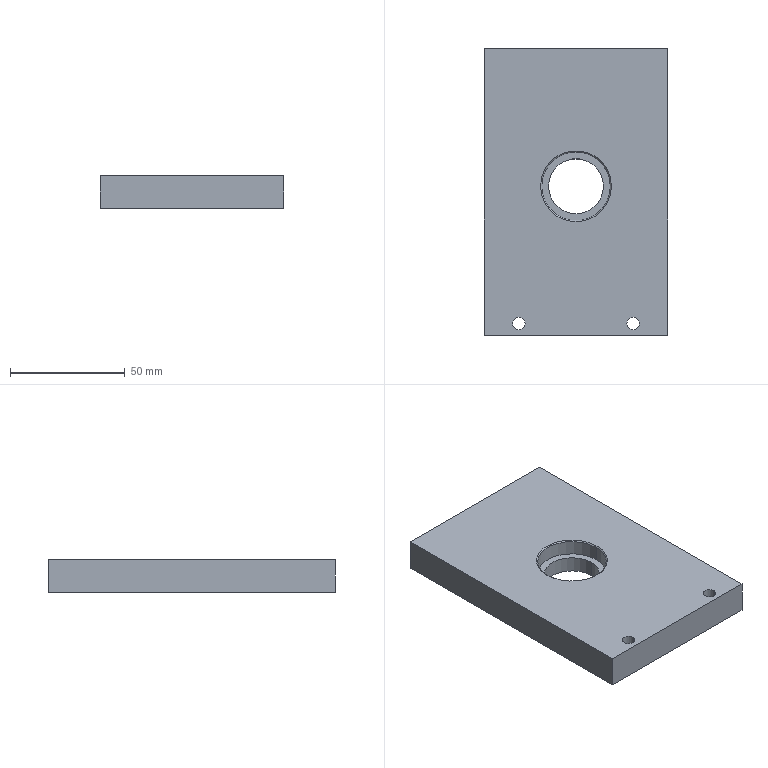Part | SolidWorks | features ICE 3, Chamfer 1, Extrusion 1, HoleWzd 1 | 1 solid | 25 faces | box 80 x 125 x 14 mm | volume 129543 mm3 | cylinder 12 | plane 7 | cone 6 | commonest cylinder face diameters 5.5 x4 6.8 x4 24 x2 30 x2
STEP:
#1=CARTESIAN_POINT('',(17.75,-120.,14.));
#2=VERTEX_POINT('',#1);
#3=CARTESIAN_POINT('',(12.25,-120.,14.));
#4=VERTEX_POINT('',#3);
#5=CARTESIAN_POINT('',(15.,-120.,14.));
#6=DIRECTION('',(0.,0.,-1.));
#7=DIRECTION('',(-1.,0.,0.));
#8=AXIS2_PLACEMENT_3D('',#5,#6,#7);
#9=CIRCLE('',#8,2.75);
#10=EDGE_CURVE('',#2,#4,#9,.T.);
#11=ORIENTED_EDGE('',*,*,#10,.F.);
#12=CARTESIAN_POINT('',(17.75,-120.,0.));
#13=VERTEX_POINT('',#12);
#14=CARTESIAN_POINT('',(17.75,-120.,14.));
#15=DIRECTION('',(0.,0.,-1.));
#16=VECTOR('',#15,1000.);
#17=LINE('',#14,#16);
#18=EDGE_CURVE('',#2,#13,#17,.T.);
#19=ORIENTED_EDGE('',*,*,#18,.T.);
#20=CARTESIAN_POINT('',(12.25,-120.,0.));
#21=VERTEX_POINT('',#20);
#22=CARTESIAN_POINT('',(15.,-120.,0.));
#23=DIRECTION('',(0.,0.,-1.));
#24=DIRECTION('',(-1.,0.,0.));
#25=AXIS2_PLACEMENT_3D('',#22,#23,#24);
#26=CIRCLE('',#25,2.75);
#27=EDGE_CURVE('',#13,#21,#26,.T.);
#28=ORIENTED_EDGE('',*,*,#27,.T.);
#29=CARTESIAN_POINT('',(12.25,-120.,14.));
#30=DIRECTION('',(0.,0.,-1.));
#31=VECTOR('',#30,1000.);
#32=LINE('',#29,#31);
#33=EDGE_CURVE('',#4,#21,#32,.T.);
#34=ORIENTED_EDGE('',*,*,#33,.F.);
#35=EDGE_LOOP('',(#11,#19,#28,#34));
#36=FACE_OUTER_BOUND('',#35,.T.);
#37=CARTESIAN_POINT('',(15.,-120.,14.));
#38=DIRECTION('',(0.,0.,-1.));
#39=DIRECTION('',(-1.,0.,0.));
#40=AXIS2_PLACEMENT_3D('',#37,#38,#39);
#41=CYLINDRICAL_SURFACE('',#40,2.75);
#42=ADVANCED_FACE('',(#36),#41,.F.);
#43=CARTESIAN_POINT('',(67.75,-120.,14.));
#44=VERTEX_POINT('',#43);
#45=CARTESIAN_POINT('',(62.25,-120.,14.));
#46=VERTEX_POINT('',#45);
#47=CARTESIAN_POINT('',(65.,-120.,14.));
#48=DIRECTION('',(0.,0.,-1.));
#49=DIRECTION('',(-1.,0.,0.));
#50=AXIS2_PLACEMENT_3D('',#47,#48,#49);
#51=CIRCLE('',#50,2.75);
#52=EDGE_CURVE('',#44,#46,#51,.T.);
#53=ORIENTED_EDGE('',*,*,#52,.F.);
#54=CARTESIAN_POINT('',(67.75,-120.,0.));
#55=VERTEX_POINT('',#54);
#56=CARTESIAN_POINT('',(67.75,-120.,14.));
#57=DIRECTION('',(0.,0.,-1.));
#58=VECTOR('',#57,1000.);
#59=LINE('',#56,#58);
#60=EDGE_CURVE('',#44,#55,#59,.T.);
#61=ORIENTED_EDGE('',*,*,#60,.T.);
#62=CARTESIAN_POINT('',(62.25,-120.,0.));
#63=VERTEX_POINT('',#62);
#64=CARTESIAN_POINT('',(65.,-120.,0.));
#65=DIRECTION('',(0.,0.,-1.));
#66=DIRECTION('',(-1.,0.,0.));
#67=AXIS2_PLACEMENT_3D('',#64,#65,#66);
#68=CIRCLE('',#67,2.75);
#69=EDGE_CURVE('',#55,#63,#68,.T.);
#70=ORIENTED_EDGE('',*,*,#69,.T.);
#71=CARTESIAN_POINT('',(62.25,-120.,14.));
#72=DIRECTION('',(0.,0.,-1.));
#73=VECTOR('',#72,1000.);
#74=LINE('',#71,#73);
#75=EDGE_CURVE('',#46,#63,#74,.T.);
#76=ORIENTED_EDGE('',*,*,#75,.F.);
#77=EDGE_LOOP('',(#53,#61,#70,#76));
#78=FACE_OUTER_BOUND('',#77,.T.);
#79=CARTESIAN_POINT('',(65.,-120.,14.));
#80=DIRECTION('',(0.,0.,-1.));
#81=DIRECTION('',(-1.,0.,0.));
#82=AXIS2_PLACEMENT_3D('',#79,#80,#81);
#83=CYLINDRICAL_SURFACE('',#82,2.75);
#84=ADVANCED_FACE('',(#78),#83,.F.);
#85=CARTESIAN_POINT('',(67.5,-22.25,3.6));
#86=VERTEX_POINT('',#85);
#87=CARTESIAN_POINT('',(67.5,-22.25,10.4));
#88=VERTEX_POINT('',#87);
#89=CARTESIAN_POINT('',(67.5,-22.25,7.));
#90=DIRECTION('',(0.,1.,0.));
#91=DIRECTION('',(0.,0.,1.));
#92=AXIS2_PLACEMENT_3D('',#89,#90,#91);
#93=CIRCLE('',#92,3.4);
#94=EDGE_CURVE('',#86,#88,#93,.T.);
#95=ORIENTED_EDGE('',*,*,#94,.F.);
#96=CARTESIAN_POINT('',(67.5,0.,3.6));
#97=VERTEX_POINT('',#96);
#98=CARTESIAN_POINT('',(67.5,0.,3.6));
#99=DIRECTION('',(0.,1.,0.));
#100=VECTOR('',#99,1000.);
#101=LINE('',#98,#100);
#102=EDGE_CURVE('',#86,#97,#101,.T.);
#103=ORIENTED_EDGE('',*,*,#102,.T.);
#104=CARTESIAN_POINT('',(67.5,0.,10.4));
#105=VERTEX_POINT('',#104);
#106=CARTESIAN_POINT('',(67.5,0.,7.));
#107=DIRECTION('',(0.,1.,0.));
#108=DIRECTION('',(0.,0.,1.));
#109=AXIS2_PLACEMENT_3D('',#106,#107,#108);
#110=CIRCLE('',#109,3.4);
#111=EDGE_CURVE('',#97,#105,#110,.T.);
#112=ORIENTED_EDGE('',*,*,#111,.T.);
#113=CARTESIAN_POINT('',(67.5,0.,10.4));
#114=DIRECTION('',(0.,1.,0.));
#115=VECTOR('',#114,1000.);
#116=LINE('',#113,#115);
#117=EDGE_CURVE('',#88,#105,#116,.T.);
#118=ORIENTED_EDGE('',*,*,#117,.F.);
#119=EDGE_LOOP('',(#95,#103,#112,#118));
#120=FACE_OUTER_BOUND('',#119,.T.);
#121=CARTESIAN_POINT('',(67.5,0.,7.));
#122=DIRECTION('',(0.,1.,0.));
#123=DIRECTION('',(0.,0.,1.));
#124=AXIS2_PLACEMENT_3D('',#121,#122,#123);
#125=CYLINDRICAL_SURFACE('',#124,3.4);
#126=ADVANCED_FACE('',(#120),#125,.F.);
#127=CARTESIAN_POINT('',(67.5,-24.293,7.));
#128=VERTEX_POINT('',#127);
#129=CARTESIAN_POINT('',(67.5,-22.25,10.4));
#130=DIRECTION('',(0.,0.515,0.8572));
#131=VECTOR('',#130,1000.);
#132=LINE('',#129,#131);
#133=EDGE_CURVE('',#128,#88,#132,.T.);
#134=ORIENTED_EDGE('',*,*,#133,.F.);
#135=CARTESIAN_POINT('',(67.5,-22.25,3.6));
#136=DIRECTION('',(0.,0.515,-0.8572));
#137=VECTOR('',#136,1000.);
#138=LINE('',#135,#137);
#139=EDGE_CURVE('',#128,#86,#138,.T.);
#140=ORIENTED_EDGE('',*,*,#139,.T.);
#141=ORIENTED_EDGE('',*,*,#94,.T.);
#142=EDGE_LOOP('',(#134,#140,#141));
#143=FACE_OUTER_BOUND('',#142,.T.);
#144=CARTESIAN_POINT('',(67.5,-22.25,7.));
#145=DIRECTION('',(0.,1.,0.));
#146=DIRECTION('',(0.,0.,1.));
#147=AXIS2_PLACEMENT_3D('',#144,#145,#146);
#148=CONICAL_SURFACE('',#147,3.4,1.03);
#149=ADVANCED_FACE('',(#143),#148,.F.);
#150=CARTESIAN_POINT('',(12.5,-22.25,3.6));
#151=VERTEX_POINT('',#150);
#152=CARTESIAN_POINT('',(12.5,-22.25,10.4));
#153=VERTEX_POINT('',#152);
#154=CARTESIAN_POINT('',(12.5,-22.25,7.));
#155=DIRECTION('',(0.,1.,0.));
#156=DIRECTION('',(0.,0.,1.));
#157=AXIS2_PLACEMENT_3D('',#154,#155,#156);
#158=CIRCLE('',#157,3.4);
#159=EDGE_CURVE('',#151,#153,#158,.T.);
#160=ORIENTED_EDGE('',*,*,#159,.F.);
#161=CARTESIAN_POINT('',(12.5,0.,3.6));
#162=VERTEX_POINT('',#161);
#163=CARTESIAN_POINT('',(12.5,0.,3.6));
#164=DIRECTION('',(0.,1.,0.));
#165=VECTOR('',#164,1000.);
#166=LINE('',#163,#165);
#167=EDGE_CURVE('',#151,#162,#166,.T.);
#168=ORIENTED_EDGE('',*,*,#167,.T.);
#169=CARTESIAN_POINT('',(12.5,0.,10.4));
#170=VERTEX_POINT('',#169);
#171=CARTESIAN_POINT('',(12.5,0.,7.));
#172=DIRECTION('',(0.,1.,0.));
#173=DIRECTION('',(0.,0.,1.));
#174=AXIS2_PLACEMENT_3D('',#171,#172,#173);
#175=CIRCLE('',#174,3.4);
#176=EDGE_CURVE('',#162,#170,#175,.T.);
#177=ORIENTED_EDGE('',*,*,#176,.T.);
#178=CARTESIAN_POINT('',(12.5,0.,10.4));
#179=DIRECTION('',(0.,1.,0.));
#180=VECTOR('',#179,1000.);
#181=LINE('',#178,#180);
#182=EDGE_CURVE('',#153,#170,#181,.T.);
#183=ORIENTED_EDGE('',*,*,#182,.F.);
#184=EDGE_LOOP('',(#160,#168,#177,#183));
#185=FACE_OUTER_BOUND('',#184,.T.);
#186=CARTESIAN_POINT('',(12.5,0.,7.));
#187=DIRECTION('',(0.,1.,0.));
#188=DIRECTION('',(0.,0.,1.));
#189=AXIS2_PLACEMENT_3D('',#186,#187,#188);
#190=CYLINDRICAL_SURFACE('',#189,3.4);
#191=ADVANCED_FACE('',(#185),#190,.F.);
#192=CARTESIAN_POINT('',(12.5,-24.293,7.));
#193=VERTEX_POINT('',#192);
#194=CARTESIAN_POINT('',(12.5,-22.25,10.4));
#195=DIRECTION('',(0.,0.515,0.8572));
#196=VECTOR('',#195,1000.);
#197=LINE('',#194,#196);
#198=EDGE_CURVE('',#193,#153,#197,.T.);
#199=ORIENTED_EDGE('',*,*,#198,.F.);
#200=CARTESIAN_POINT('',(12.5,-22.25,3.6));
#201=DIRECTION('',(0.,0.515,-0.8572));
#202=VECTOR('',#201,1000.);
#203=LINE('',#200,#202);
#204=EDGE_CURVE('',#193,#151,#203,.T.);
#205=ORIENTED_EDGE('',*,*,#204,.T.);
#206=ORIENTED_EDGE('',*,*,#159,.T.);
#207=EDGE_LOOP('',(#199,#205,#206));
#208=FACE_OUTER_BOUND('',#207,.T.);
#209=CARTESIAN_POINT('',(12.5,-22.25,7.));
#210=DIRECTION('',(0.,1.,0.));
#211=DIRECTION('',(0.,0.,1.));
#212=AXIS2_PLACEMENT_3D('',#209,#210,#211);
#213=CONICAL_SURFACE('',#212,3.4,1.03);
#214=ADVANCED_FACE('',(#208),#213,.F.);
#215=CARTESIAN_POINT('',(25.,-60.,13.5));
#216=VERTEX_POINT('',#215);
#217=CARTESIAN_POINT('',(55.,-60.,13.5));
#218=VERTEX_POINT('',#217);
#219=CARTESIAN_POINT('',(40.,-60.,13.5));
#220=DIRECTION('',(0.,0.,1.));
#221=DIRECTION('',(1.,0.,0.));
#222=AXIS2_PLACEMENT_3D('',#219,#220,#221);
#223=CIRCLE('',#222,15.);
#224=EDGE_CURVE('',#216,#218,#223,.T.);
#225=ORIENTED_EDGE('',*,*,#224,.F.);
#226=CARTESIAN_POINT('',(24.5,-60.,14.));
#227=VERTEX_POINT('',#226);
#228=CARTESIAN_POINT('',(25.,-60.,13.5));
#229=DIRECTION('',(-0.7071,0.,0.7071));
#230=VECTOR('',#229,1000.);
#231=LINE('',#228,#230);
#232=EDGE_CURVE('',#216,#227,#231,.T.);
#233=ORIENTED_EDGE('',*,*,#232,.T.);
#234=CARTESIAN_POINT('',(55.5,-60.,14.));
#235=VERTEX_POINT('',#234);
#236=CARTESIAN_POINT('',(40.,-60.,14.));
#237=DIRECTION('',(0.,0.,-1.));
#238=DIRECTION('',(1.,0.,0.));
#239=AXIS2_PLACEMENT_3D('',#236,#237,#238);
#240=CIRCLE('',#239,15.5);
#241=EDGE_CURVE('',#235,#227,#240,.T.);
#242=ORIENTED_EDGE('',*,*,#241,.F.);
#243=CARTESIAN_POINT('',(55.,-60.,13.5));
#244=DIRECTION('',(0.7071,0.,0.7071));
#245=VECTOR('',#244,1000.);
#246=LINE('',#243,#245);
#247=EDGE_CURVE('',#218,#235,#246,.T.);
#248=ORIENTED_EDGE('',*,*,#247,.F.);
#249=EDGE_LOOP('',(#225,#233,#242,#248));
#250=FACE_OUTER_BOUND('',#249,.T.);
#251=CARTESIAN_POINT('',(40.,-60.,13.5));
#252=DIRECTION('',(0.,0.,1.));
#253=DIRECTION('',(1.,0.,0.));
#254=AXIS2_PLACEMENT_3D('',#251,#252,#253);
#255=CONICAL_SURFACE('',#254,15.,0.7854);
#256=ADVANCED_FACE('',(#250),#255,.F.);
#257=CARTESIAN_POINT('',(28.,-60.,0.));
#258=VERTEX_POINT('',#257);
#259=CARTESIAN_POINT('',(52.,-60.,0.));
#260=VERTEX_POINT('',#259);
#261=CARTESIAN_POINT('',(40.,-60.,0.));
#262=DIRECTION('',(0.,0.,1.));
#263=DIRECTION('',(1.,0.,0.));
#264=AXIS2_PLACEMENT_3D('',#261,#262,#263);
#265=CIRCLE('',#264,12.);
#266=EDGE_CURVE('',#258,#260,#265,.T.);
#267=ORIENTED_EDGE('',*,*,#266,.F.);
#268=CARTESIAN_POINT('',(28.,-60.,7.));
#269=VERTEX_POINT('',#268);
#270=CARTESIAN_POINT('',(28.,-60.,0.));
#271=DIRECTION('',(0.,0.,1.));
#272=VECTOR('',#271,1000.);
#273=LINE('',#270,#272);
#274=EDGE_CURVE('',#258,#269,#273,.T.);
#275=ORIENTED_EDGE('',*,*,#274,.T.);
#276=CARTESIAN_POINT('',(52.,-60.,7.));
#277=VERTEX_POINT('',#276);
#278=CARTESIAN_POINT('',(40.,-60.,7.));
#279=DIRECTION('',(0.,0.,1.));
#280=DIRECTION('',(1.,0.,0.));
#281=AXIS2_PLACEMENT_3D('',#278,#279,#280);
#282=CIRCLE('',#281,12.);
#283=EDGE_CURVE('',#269,#277,#282,.T.);
#284=ORIENTED_EDGE('',*,*,#283,.T.);
#285=CARTESIAN_POINT('',(52.,-60.,0.));
#286=DIRECTION('',(0.,0.,1.));
#287=VECTOR('',#286,1000.);
#288=LINE('',#285,#287);
#289=EDGE_CURVE('',#260,#277,#288,.T.);
#290=ORIENTED_EDGE('',*,*,#289,.F.);
#291=EDGE_LOOP('',(#267,#275,#284,#290));
#292=FACE_OUTER_BOUND('',#291,.T.);
#293=CARTESIAN_POINT('',(40.,-60.,0.));
#294=DIRECTION('',(0.,0.,1.));
#295=DIRECTION('',(1.,0.,0.));
#296=AXIS2_PLACEMENT_3D('',#293,#294,#295);
#297=CYLINDRICAL_SURFACE('',#296,12.);
#298=ADVANCED_FACE('',(#292),#297,.F.);
#299=CARTESIAN_POINT('',(25.,-60.,7.));
#300=VERTEX_POINT('',#299);
#301=CARTESIAN_POINT('',(55.,-60.,7.));
#302=VERTEX_POINT('',#301);
#303=CARTESIAN_POINT('',(40.,-60.,7.));
#304=DIRECTION('',(0.,0.,1.));
#305=DIRECTION('',(1.,0.,0.));
#306=AXIS2_PLACEMENT_3D('',#303,#304,#305);
#307=CIRCLE('',#306,15.);
#308=EDGE_CURVE('',#300,#302,#307,.T.);
#309=ORIENTED_EDGE('',*,*,#308,.F.);
#310=CARTESIAN_POINT('',(25.,-60.,7.));
#311=DIRECTION('',(0.,0.,1.));
#312=VECTOR('',#311,1000.);
#313=LINE('',#310,#312);
#314=EDGE_CURVE('',#300,#216,#313,.T.);
#315=ORIENTED_EDGE('',*,*,#314,.T.);
#316=ORIENTED_EDGE('',*,*,#224,.T.);
#317=CARTESIAN_POINT('',(55.,-60.,7.));
#318=DIRECTION('',(0.,0.,1.));
#319=VECTOR('',#318,1000.);
#320=LINE('',#317,#319);
#321=EDGE_CURVE('',#302,#218,#320,.T.);
#322=ORIENTED_EDGE('',*,*,#321,.F.);
#323=EDGE_LOOP('',(#309,#315,#316,#322));
#324=FACE_OUTER_BOUND('',#323,.T.);
#325=CARTESIAN_POINT('',(40.,-60.,7.));
#326=DIRECTION('',(0.,0.,1.));
#327=DIRECTION('',(1.,0.,0.));
#328=AXIS2_PLACEMENT_3D('',#325,#326,#327);
#329=CYLINDRICAL_SURFACE('',#328,15.);
#330=ADVANCED_FACE('',(#324),#329,.F.);
#331=CARTESIAN_POINT('',(0.,0.,0.));
#332=VERTEX_POINT('',#331);
#333=CARTESIAN_POINT('',(0.,-125.,0.));
#334=VERTEX_POINT('',#333);
#335=CARTESIAN_POINT('',(0.,0.,0.));
#336=DIRECTION('',(0.,-1.,0.));
#337=VECTOR('',#336,1000.);
#338=LINE('',#335,#337);
#339=EDGE_CURVE('',#332,#334,#338,.T.);
#340=ORIENTED_EDGE('',*,*,#339,.T.);
#341=CARTESIAN_POINT('',(0.,-125.,14.));
#342=VERTEX_POINT('',#341);
#343=CARTESIAN_POINT('',(0.,-125.,14.));
#344=DIRECTION('',(0.,0.,-1.));
#345=VECTOR('',#344,1000.);
#346=LINE('',#343,#345);
#347=EDGE_CURVE('',#342,#334,#346,.T.);
#348=ORIENTED_EDGE('',*,*,#347,.F.);
#349=CARTESIAN_POINT('',(0.,0.,14.));
#350=VERTEX_POINT('',#349);
#351=CARTESIAN_POINT('',(0.,0.,14.));
#352=DIRECTION('',(0.,-1.,0.));
#353=VECTOR('',#352,1000.);
#354=LINE('',#351,#353);
#355=EDGE_CURVE('',#350,#342,#354,.T.);
#356=ORIENTED_EDGE('',*,*,#355,.F.);
#357=CARTESIAN_POINT('',(0.,0.,14.));
#358=DIRECTION('',(0.,0.,-1.));
#359=VECTOR('',#358,1000.);
#360=LINE('',#357,#359);
#361=EDGE_CURVE('',#350,#332,#360,.T.);
#362=ORIENTED_EDGE('',*,*,#361,.T.);
#363=EDGE_LOOP('',(#340,#348,#356,#362));
#364=FACE_OUTER_BOUND('',#363,.T.);
#365=CARTESIAN_POINT('',(0.,0.,14.));
#366=DIRECTION('',(1.,0.,0.));
#367=DIRECTION('',(0.,1.,0.));
#368=AXIS2_PLACEMENT_3D('',#365,#366,#367);
#369=PLANE('',#368);
#370=ADVANCED_FACE('',(#364),#369,.F.);
#371=CARTESIAN_POINT('',(80.,-125.,0.));
#372=VERTEX_POINT('',#371);
#373=CARTESIAN_POINT('',(0.,-125.,0.));
#374=DIRECTION('',(1.,0.,0.));
#375=VECTOR('',#374,1000.);
#376=LINE('',#373,#375);
#377=EDGE_CURVE('',#334,#372,#376,.T.);
#378=ORIENTED_EDGE('',*,*,#377,.T.);
#379=CARTESIAN_POINT('',(80.,-125.,14.));
#380=VERTEX_POINT('',#379);
#381=CARTESIAN_POINT('',(80.,-125.,14.));
#382=DIRECTION('',(0.,0.,-1.));
#383=VECTOR('',#382,1000.);
#384=LINE('',#381,#383);
#385=EDGE_CURVE('',#380,#372,#384,.T.);
#386=ORIENTED_EDGE('',*,*,#385,.F.);
#387=CARTESIAN_POINT('',(0.,-125.,14.));
#388=DIRECTION('',(1.,0.,0.));
#389=VECTOR('',#388,1000.);
#390=LINE('',#387,#389);
#391=EDGE_CURVE('',#342,#380,#390,.T.);
#392=ORIENTED_EDGE('',*,*,#391,.F.);
#393=ORIENTED_EDGE('',*,*,#347,.T.);
#394=EDGE_LOOP('',(#378,#386,#392,#393));
#395=FACE_OUTER_BOUND('',#394,.T.);
#396=CARTESIAN_POINT('',(0.,-125.,14.));
#397=DIRECTION('',(0.,1.,0.));
#398=DIRECTION('',(0.,0.,1.));
#399=AXIS2_PLACEMENT_3D('',#396,#397,#398);
#400=PLANE('',#399);
#401=ADVANCED_FACE('',(#395),#400,.F.);
#402=CARTESIAN_POINT('',(80.,0.,0.));
#403=VERTEX_POINT('',#402);
#404=CARTESIAN_POINT('',(80.,0.,0.));
#405=DIRECTION('',(0.,1.,0.));
#406=VECTOR('',#405,1000.);
#407=LINE('',#404,#406);
#408=EDGE_CURVE('',#372,#403,#407,.T.);
#409=ORIENTED_EDGE('',*,*,#408,.T.);
#410=CARTESIAN_POINT('',(80.,0.,14.));
#411=VERTEX_POINT('',#410);
#412=CARTESIAN_POINT('',(80.,0.,14.));
#413=DIRECTION('',(0.,0.,-1.));
#414=VECTOR('',#413,1000.);
#415=LINE('',#412,#414);
#416=EDGE_CURVE('',#411,#403,#415,.T.);
#417=ORIENTED_EDGE('',*,*,#416,.F.);
#418=CARTESIAN_POINT('',(80.,0.,14.));
#419=DIRECTION('',(0.,1.,0.));
#420=VECTOR('',#419,1000.);
#421=LINE('',#418,#420);
#422=EDGE_CURVE('',#380,#411,#421,.T.);
#423=ORIENTED_EDGE('',*,*,#422,.F.);
#424=ORIENTED_EDGE('',*,*,#385,.T.);
#425=EDGE_LOOP('',(#409,#417,#423,#424));
#426=FACE_OUTER_BOUND('',#425,.T.);
#427=CARTESIAN_POINT('',(80.,0.,14.));
#428=DIRECTION('',(-1.,0.,0.));
#429=DIRECTION('',(0.,-1.,0.));
#430=AXIS2_PLACEMENT_3D('',#427,#428,#429);
#431=PLANE('',#430);
#432=ADVANCED_FACE('',(#426),#431,.F.);
#433=CARTESIAN_POINT('',(67.5,0.,7.));
#434=DIRECTION('',(0.,1.,0.));
#435=DIRECTION('',(0.,0.,1.));
#436=AXIS2_PLACEMENT_3D('',#433,#434,#435);
#437=CIRCLE('',#436,3.4);
#438=EDGE_CURVE('',#105,#97,#437,.T.);
#439=ORIENTED_EDGE('',*,*,#438,.F.);
#440=ORIENTED_EDGE('',*,*,#111,.F.);
#441=EDGE_LOOP('',(#439,#440));
#442=FACE_BOUND('',#441,.T.);
#443=CARTESIAN_POINT('',(12.5,0.,7.));
#444=DIRECTION('',(0.,1.,0.));
#445=DIRECTION('',(0.,0.,1.));
#446=AXIS2_PLACEMENT_3D('',#443,#444,#445);
#447=CIRCLE('',#446,3.4);
#448=EDGE_CURVE('',#170,#162,#447,.T.);
#449=ORIENTED_EDGE('',*,*,#448,.F.);
#450=ORIENTED_EDGE('',*,*,#176,.F.);
#451=EDGE_LOOP('',(#449,#450));
#452=FACE_BOUND('',#451,.T.);
#453=CARTESIAN_POINT('',(0.,0.,0.));
#454=DIRECTION('',(-1.,0.,0.));
#455=VECTOR('',#454,1000.);
#456=LINE('',#453,#455);
#457=EDGE_CURVE('',#403,#332,#456,.T.);
#458=ORIENTED_EDGE('',*,*,#457,.T.);
#459=ORIENTED_EDGE('',*,*,#361,.F.);
#460=CARTESIAN_POINT('',(0.,0.,14.));
#461=DIRECTION('',(-1.,0.,0.));
#462=VECTOR('',#461,1000.);
#463=LINE('',#460,#462);
#464=EDGE_CURVE('',#411,#350,#463,.T.);
#465=ORIENTED_EDGE('',*,*,#464,.F.);
#466=ORIENTED_EDGE('',*,*,#416,.T.);
#467=EDGE_LOOP('',(#458,#459,#465,#466));
#468=FACE_OUTER_BOUND('',#467,.T.);
#469=CARTESIAN_POINT('',(0.,0.,14.));
#470=DIRECTION('',(0.,-1.,0.));
#471=DIRECTION('',(0.,0.,-1.));
#472=AXIS2_PLACEMENT_3D('',#469,#470,#471);
#473=PLANE('',#472);
#474=ADVANCED_FACE('',(#442,#452,#468),#473,.F.);
#475=CARTESIAN_POINT('',(15.,-120.,14.));
#476=DIRECTION('',(0.,0.,-1.));
#477=DIRECTION('',(-1.,0.,0.));
#478=AXIS2_PLACEMENT_3D('',#475,#476,#477);
#479=CIRCLE('',#478,2.75);
#480=EDGE_CURVE('',#4,#2,#479,.T.);
#481=ORIENTED_EDGE('',*,*,#480,.T.);
#482=ORIENTED_EDGE('',*,*,#10,.T.);
#483=EDGE_LOOP('',(#481,#482));
#484=FACE_BOUND('',#483,.T.);
#485=CARTESIAN_POINT('',(65.,-120.,14.));
#486=DIRECTION('',(0.,0.,-1.));
#487=DIRECTION('',(-1.,0.,0.));
#488=AXIS2_PLACEMENT_3D('',#485,#486,#487);
#489=CIRCLE('',#488,2.75);
#490=EDGE_CURVE('',#46,#44,#489,.T.);
#491=ORIENTED_EDGE('',*,*,#490,.T.);
#492=ORIENTED_EDGE('',*,*,#52,.T.);
#493=EDGE_LOOP('',(#491,#492));
#494=FACE_BOUND('',#493,.T.);
#495=ORIENTED_EDGE('',*,*,#241,.T.);
#496=CARTESIAN_POINT('',(40.,-60.,14.));
#497=DIRECTION('',(0.,0.,-1.));
#498=DIRECTION('',(1.,0.,0.));
#499=AXIS2_PLACEMENT_3D('',#496,#497,#498);
#500=CIRCLE('',#499,15.5);
#501=EDGE_CURVE('',#227,#235,#500,.T.);
#502=ORIENTED_EDGE('',*,*,#501,.T.);
#503=EDGE_LOOP('',(#495,#502));
#504=FACE_BOUND('',#503,.T.);
#505=ORIENTED_EDGE('',*,*,#355,.T.);
#506=ORIENTED_EDGE('',*,*,#391,.T.);
#507=ORIENTED_EDGE('',*,*,#422,.T.);
#508=ORIENTED_EDGE('',*,*,#464,.T.);
#509=EDGE_LOOP('',(#505,#506,#507,#508));
#510=FACE_OUTER_BOUND('',#509,.T.);
#511=CARTESIAN_POINT('',(0.,0.,14.));
#512=DIRECTION('',(0.,0.,1.));
#513=DIRECTION('',(1.,0.,0.));
#514=AXIS2_PLACEMENT_3D('',#511,#512,#513);
#515=PLANE('',#514);
#516=ADVANCED_FACE('',(#484,#494,#504,#510),#515,.T.);
#517=CARTESIAN_POINT('',(15.,-120.,0.));
#518=DIRECTION('',(0.,0.,-1.));
#519=DIRECTION('',(-1.,0.,0.));
#520=AXIS2_PLACEMENT_3D('',#517,#518,#519);
#521=CIRCLE('',#520,2.75);
#522=EDGE_CURVE('',#21,#13,#521,.T.);
#523=ORIENTED_EDGE('',*,*,#522,.F.);
#524=ORIENTED_EDGE('',*,*,#27,.F.);
#525=EDGE_LOOP('',(#523,#524));
#526=FACE_BOUND('',#525,.T.);
#527=CARTESIAN_POINT('',(65.,-120.,0.));
#528=DIRECTION('',(0.,0.,-1.));
#529=DIRECTION('',(-1.,0.,0.));
#530=AXIS2_PLACEMENT_3D('',#527,#528,#529);
#531=CIRCLE('',#530,2.75);
#532=EDGE_CURVE('',#63,#55,#531,.T.);
#533=ORIENTED_EDGE('',*,*,#532,.F.);
#534=ORIENTED_EDGE('',*,*,#69,.F.);
#535=EDGE_LOOP('',(#533,#534));
#536=FACE_BOUND('',#535,.T.);
#537=CARTESIAN_POINT('',(40.,-60.,0.));
#538=DIRECTION('',(0.,0.,1.));
#539=DIRECTION('',(1.,0.,0.));
#540=AXIS2_PLACEMENT_3D('',#537,#538,#539);
#541=CIRCLE('',#540,12.);
#542=EDGE_CURVE('',#260,#258,#541,.T.);
#543=ORIENTED_EDGE('',*,*,#542,.T.);
#544=ORIENTED_EDGE('',*,*,#266,.T.);
#545=EDGE_LOOP('',(#543,#544));
#546=FACE_BOUND('',#545,.T.);
#547=ORIENTED_EDGE('',*,*,#339,.F.);
#548=ORIENTED_EDGE('',*,*,#457,.F.);
#549=ORIENTED_EDGE('',*,*,#408,.F.);
#550=ORIENTED_EDGE('',*,*,#377,.F.);
#551=EDGE_LOOP('',(#547,#548,#549,#550));
#552=FACE_OUTER_BOUND('',#551,.T.);
#553=CARTESIAN_POINT('',(0.,0.,0.));
#554=DIRECTION('',(0.,0.,1.));
#555=DIRECTION('',(1.,0.,0.));
#556=AXIS2_PLACEMENT_3D('',#553,#554,#555);
#557=PLANE('',#556);
#558=ADVANCED_FACE('',(#526,#536,#546,#552),#557,.F.);
#559=ORIENTED_EDGE('',*,*,#314,.F.);
#560=CARTESIAN_POINT('',(40.,-60.,7.));
#561=DIRECTION('',(0.,0.,1.));
#562=DIRECTION('',(1.,0.,0.));
#563=AXIS2_PLACEMENT_3D('',#560,#561,#562);
#564=CIRCLE('',#563,15.);
#565=EDGE_CURVE('',#302,#300,#564,.T.);
#566=ORIENTED_EDGE('',*,*,#565,.F.);
#567=ORIENTED_EDGE('',*,*,#321,.T.);
#568=CARTESIAN_POINT('',(40.,-60.,13.5));
#569=DIRECTION('',(0.,0.,1.));
#570=DIRECTION('',(1.,0.,0.));
#571=AXIS2_PLACEMENT_3D('',#568,#569,#570);
#572=CIRCLE('',#571,15.);
#573=EDGE_CURVE('',#218,#216,#572,.T.);
#574=ORIENTED_EDGE('',*,*,#573,.T.);
#575=EDGE_LOOP('',(#559,#566,#567,#574));
#576=FACE_OUTER_BOUND('',#575,.T.);
#577=CARTESIAN_POINT('',(40.,-60.,7.));
#578=DIRECTION('',(0.,0.,1.));
#579=DIRECTION('',(1.,0.,0.));
#580=AXIS2_PLACEMENT_3D('',#577,#578,#579);
#581=CYLINDRICAL_SURFACE('',#580,15.);
#582=ADVANCED_FACE('',(#576),#581,.F.);
#583=CARTESIAN_POINT('',(40.,-60.,7.));
#584=DIRECTION('',(0.,0.,1.));
#585=DIRECTION('',(1.,0.,0.));
#586=AXIS2_PLACEMENT_3D('',#583,#584,#585);
#587=CIRCLE('',#586,12.);
#588=EDGE_CURVE('',#277,#269,#587,.T.);
#589=ORIENTED_EDGE('',*,*,#588,.F.);
#590=ORIENTED_EDGE('',*,*,#283,.F.);
#591=EDGE_LOOP('',(#589,#590));
#592=FACE_BOUND('',#591,.T.);
#593=ORIENTED_EDGE('',*,*,#565,.T.);
#594=ORIENTED_EDGE('',*,*,#308,.T.);
#595=EDGE_LOOP('',(#593,#594));
#596=FACE_OUTER_BOUND('',#595,.T.);
#597=CARTESIAN_POINT('',(40.,-60.,7.));
#598=DIRECTION('',(0.,0.,1.));
#599=DIRECTION('',(1.,0.,0.));
#600=AXIS2_PLACEMENT_3D('',#597,#598,#599);
#601=PLANE('',#600);
#602=ADVANCED_FACE('',(#592,#596),#601,.T.);
#603=ORIENTED_EDGE('',*,*,#274,.F.);
#604=ORIENTED_EDGE('',*,*,#542,.F.);
#605=ORIENTED_EDGE('',*,*,#289,.T.);
#606=ORIENTED_EDGE('',*,*,#588,.T.);
#607=EDGE_LOOP('',(#603,#604,#605,#606));
#608=FACE_OUTER_BOUND('',#607,.T.);
#609=CARTESIAN_POINT('',(40.,-60.,0.));
#610=DIRECTION('',(0.,0.,1.));
#611=DIRECTION('',(1.,0.,0.));
#612=AXIS2_PLACEMENT_3D('',#609,#610,#611);
#613=CYLINDRICAL_SURFACE('',#612,12.);
#614=ADVANCED_FACE('',(#608),#613,.F.);
#615=ORIENTED_EDGE('',*,*,#232,.F.);
#616=ORIENTED_EDGE('',*,*,#573,.F.);
#617=ORIENTED_EDGE('',*,*,#247,.T.);
#618=ORIENTED_EDGE('',*,*,#501,.F.);
#619=EDGE_LOOP('',(#615,#616,#617,#618));
#620=FACE_OUTER_BOUND('',#619,.T.);
#621=CARTESIAN_POINT('',(40.,-60.,13.5));
#622=DIRECTION('',(0.,0.,1.));
#623=DIRECTION('',(1.,0.,0.));
#624=AXIS2_PLACEMENT_3D('',#621,#622,#623);
#625=CONICAL_SURFACE('',#624,15.,0.7854);
#626=ADVANCED_FACE('',(#620),#625,.F.);
#627=ORIENTED_EDGE('',*,*,#204,.F.);
#628=ORIENTED_EDGE('',*,*,#198,.T.);
#629=CARTESIAN_POINT('',(12.5,-22.25,7.));
#630=DIRECTION('',(0.,1.,0.));
#631=DIRECTION('',(0.,0.,1.));
#632=AXIS2_PLACEMENT_3D('',#629,#630,#631);
#633=CIRCLE('',#632,3.4);
#634=EDGE_CURVE('',#153,#151,#633,.T.);
#635=ORIENTED_EDGE('',*,*,#634,.T.);
#636=EDGE_LOOP('',(#627,#628,#635));
#637=FACE_OUTER_BOUND('',#636,.T.);
#638=CARTESIAN_POINT('',(12.5,-22.25,7.));
#639=DIRECTION('',(0.,1.,0.));
#640=DIRECTION('',(0.,0.,1.));
#641=AXIS2_PLACEMENT_3D('',#638,#639,#640);
#642=CONICAL_SURFACE('',#641,3.4,1.03);
#643=ADVANCED_FACE('',(#637),#642,.F.);
#644=ORIENTED_EDGE('',*,*,#167,.F.);
#645=ORIENTED_EDGE('',*,*,#634,.F.);
#646=ORIENTED_EDGE('',*,*,#182,.T.);
#647=ORIENTED_EDGE('',*,*,#448,.T.);
#648=EDGE_LOOP('',(#644,#645,#646,#647));
#649=FACE_OUTER_BOUND('',#648,.T.);
#650=CARTESIAN_POINT('',(12.5,0.,7.));
#651=DIRECTION('',(0.,1.,0.));
#652=DIRECTION('',(0.,0.,1.));
#653=AXIS2_PLACEMENT_3D('',#650,#651,#652);
#654=CYLINDRICAL_SURFACE('',#653,3.4);
#655=ADVANCED_FACE('',(#649),#654,.F.);
#656=ORIENTED_EDGE('',*,*,#139,.F.);
#657=ORIENTED_EDGE('',*,*,#133,.T.);
#658=CARTESIAN_POINT('',(67.5,-22.25,7.));
#659=DIRECTION('',(0.,1.,0.));
#660=DIRECTION('',(0.,0.,1.));
#661=AXIS2_PLACEMENT_3D('',#658,#659,#660);
#662=CIRCLE('',#661,3.4);
#663=EDGE_CURVE('',#88,#86,#662,.T.);
#664=ORIENTED_EDGE('',*,*,#663,.T.);
#665=EDGE_LOOP('',(#656,#657,#664));
#666=FACE_OUTER_BOUND('',#665,.T.);
#667=CARTESIAN_POINT('',(67.5,-22.25,7.));
#668=DIRECTION('',(0.,1.,0.));
#669=DIRECTION('',(0.,0.,1.));
#670=AXIS2_PLACEMENT_3D('',#667,#668,#669);
#671=CONICAL_SURFACE('',#670,3.4,1.03);
#672=ADVANCED_FACE('',(#666),#671,.F.);
#673=ORIENTED_EDGE('',*,*,#102,.F.);
#674=ORIENTED_EDGE('',*,*,#663,.F.);
#675=ORIENTED_EDGE('',*,*,#117,.T.);
#676=ORIENTED_EDGE('',*,*,#438,.T.);
#677=EDGE_LOOP('',(#673,#674,#675,#676));
#678=FACE_OUTER_BOUND('',#677,.T.);
#679=CARTESIAN_POINT('',(67.5,0.,7.));
#680=DIRECTION('',(0.,1.,0.));
#681=DIRECTION('',(0.,0.,1.));
#682=AXIS2_PLACEMENT_3D('',#679,#680,#681);
#683=CYLINDRICAL_SURFACE('',#682,3.4);
#684=ADVANCED_FACE('',(#678),#683,.F.);
#685=ORIENTED_EDGE('',*,*,#60,.F.);
#686=ORIENTED_EDGE('',*,*,#490,.F.);
#687=ORIENTED_EDGE('',*,*,#75,.T.);
#688=ORIENTED_EDGE('',*,*,#532,.T.);
#689=EDGE_LOOP('',(#685,#686,#687,#688));
#690=FACE_OUTER_BOUND('',#689,.T.);
#691=CARTESIAN_POINT('',(65.,-120.,14.));
#692=DIRECTION('',(0.,0.,-1.));
#693=DIRECTION('',(-1.,0.,0.));
#694=AXIS2_PLACEMENT_3D('',#691,#692,#693);
#695=CYLINDRICAL_SURFACE('',#694,2.75);
#696=ADVANCED_FACE('',(#690),#695,.F.);
#697=ORIENTED_EDGE('',*,*,#18,.F.);
#698=ORIENTED_EDGE('',*,*,#480,.F.);
#699=ORIENTED_EDGE('',*,*,#33,.T.);
#700=ORIENTED_EDGE('',*,*,#522,.T.);
#701=EDGE_LOOP('',(#697,#698,#699,#700));
#702=FACE_OUTER_BOUND('',#701,.T.);
#703=CARTESIAN_POINT('',(15.,-120.,14.));
#704=DIRECTION('',(0.,0.,-1.));
#705=DIRECTION('',(-1.,0.,0.));
#706=AXIS2_PLACEMENT_3D('',#703,#704,#705);
#707=CYLINDRICAL_SURFACE('',#706,2.75);
#708=ADVANCED_FACE('',(#702),#707,.F.);
#709=CLOSED_SHELL('',(#42,#84,#126,#149,#191,#214,#256,#298,#330,#370,#401,#432,#474,#516,#558,#582,#602,#614,#626,#643,#655,#672,#684,#696,#708));
#710=MANIFOLD_SOLID_BREP('',#709);
#711=CARTESIAN_POINT('',(0.,0.,0.));
#712=DIRECTION('',(0.,0.,1.));
#713=DIRECTION('',(1.,0.,0.));
#714=AXIS2_PLACEMENT_3D('',#711,#712,#713);
#715=(LENGTH_UNIT()NAMED_UNIT(*)SI_UNIT(.MILLI.,.METRE.));
#716=UNCERTAINTY_MEASURE_WITH_UNIT(LENGTH_MEASURE(0.00001),#715,'','');
#717=(NAMED_UNIT(*)PLANE_ANGLE_UNIT()SI_UNIT($,.RADIAN.));
#718=(NAMED_UNIT(*)SI_UNIT($,.STERADIAN.)SOLID_ANGLE_UNIT());
#719=(GEOMETRIC_REPRESENTATION_CONTEXT(3)GLOBAL_UNCERTAINTY_ASSIGNED_CONTEXT((#716))GLOBAL_UNIT_ASSIGNED_CONTEXT((#715,#717,#718))REPRESENTATION_CONTEXT('',''));
#720=ADVANCED_BREP_SHAPE_REPRESENTATION('',(#710,#714),#719);